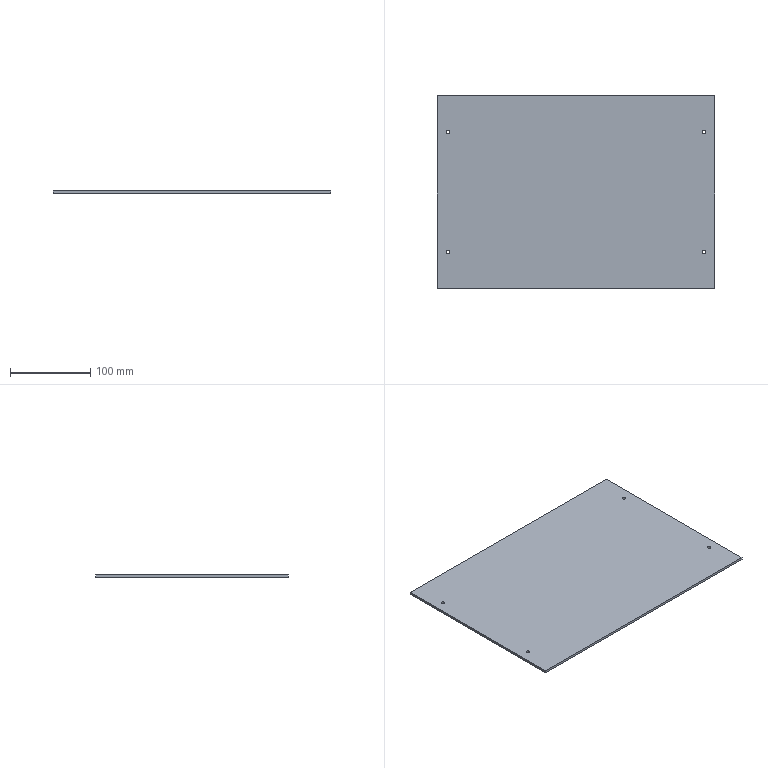Part | SolidWorks | features Cut 1, Extrusion 1 | 1 solid | 14 faces | box 346 x 240 x 3 mm | volume 248938 mm3 | cylinder 8 | plane 6 | commonest cylinder face diameters 4.4 x8
STEP:
#1=CARTESIAN_POINT('',(-162.2,-75.,0.));
#2=VERTEX_POINT('',#1);
#3=CARTESIAN_POINT('',(-157.8,-75.,0.));
#4=VERTEX_POINT('',#3);
#5=CARTESIAN_POINT('',(-160.,-75.,0.));
#6=DIRECTION('',(0.,0.,1.));
#7=DIRECTION('',(1.,0.,0.));
#8=AXIS2_PLACEMENT_3D('',#5,#6,#7);
#9=CIRCLE('',#8,2.2);
#10=EDGE_CURVE('',#2,#4,#9,.T.);
#11=ORIENTED_EDGE('',*,*,#10,.F.);
#12=CARTESIAN_POINT('',(-162.2,-75.,3.));
#13=VERTEX_POINT('',#12);
#14=CARTESIAN_POINT('',(-162.2,-75.,-7.));
#15=DIRECTION('',(0.,0.,1.));
#16=VECTOR('',#15,1000.);
#17=LINE('',#14,#16);
#18=EDGE_CURVE('',#2,#13,#17,.T.);
#19=ORIENTED_EDGE('',*,*,#18,.T.);
#20=CARTESIAN_POINT('',(-157.8,-75.,3.));
#21=VERTEX_POINT('',#20);
#22=CARTESIAN_POINT('',(-160.,-75.,3.));
#23=DIRECTION('',(0.,0.,1.));
#24=DIRECTION('',(1.,0.,0.));
#25=AXIS2_PLACEMENT_3D('',#22,#23,#24);
#26=CIRCLE('',#25,2.2);
#27=EDGE_CURVE('',#13,#21,#26,.T.);
#28=ORIENTED_EDGE('',*,*,#27,.T.);
#29=CARTESIAN_POINT('',(-157.8,-75.,-7.));
#30=DIRECTION('',(0.,0.,1.));
#31=VECTOR('',#30,1000.);
#32=LINE('',#29,#31);
#33=EDGE_CURVE('',#4,#21,#32,.T.);
#34=ORIENTED_EDGE('',*,*,#33,.F.);
#35=EDGE_LOOP('',(#11,#19,#28,#34));
#36=FACE_OUTER_BOUND('',#35,.T.);
#37=CARTESIAN_POINT('',(-160.,-75.,-7.));
#38=DIRECTION('',(0.,0.,1.));
#39=DIRECTION('',(1.,0.,0.));
#40=AXIS2_PLACEMENT_3D('',#37,#38,#39);
#41=CYLINDRICAL_SURFACE('',#40,2.2);
#42=ADVANCED_FACE('',(#36),#41,.F.);
#43=CARTESIAN_POINT('',(-162.2,75.,0.));
#44=VERTEX_POINT('',#43);
#45=CARTESIAN_POINT('',(-157.8,75.,0.));
#46=VERTEX_POINT('',#45);
#47=CARTESIAN_POINT('',(-160.,75.,0.));
#48=DIRECTION('',(0.,0.,1.));
#49=DIRECTION('',(1.,0.,0.));
#50=AXIS2_PLACEMENT_3D('',#47,#48,#49);
#51=CIRCLE('',#50,2.2);
#52=EDGE_CURVE('',#44,#46,#51,.T.);
#53=ORIENTED_EDGE('',*,*,#52,.F.);
#54=CARTESIAN_POINT('',(-162.2,75.,3.));
#55=VERTEX_POINT('',#54);
#56=CARTESIAN_POINT('',(-162.2,75.,-7.));
#57=DIRECTION('',(0.,0.,1.));
#58=VECTOR('',#57,1000.);
#59=LINE('',#56,#58);
#60=EDGE_CURVE('',#44,#55,#59,.T.);
#61=ORIENTED_EDGE('',*,*,#60,.T.);
#62=CARTESIAN_POINT('',(-157.8,75.,3.));
#63=VERTEX_POINT('',#62);
#64=CARTESIAN_POINT('',(-160.,75.,3.));
#65=DIRECTION('',(0.,0.,1.));
#66=DIRECTION('',(1.,0.,0.));
#67=AXIS2_PLACEMENT_3D('',#64,#65,#66);
#68=CIRCLE('',#67,2.2);
#69=EDGE_CURVE('',#55,#63,#68,.T.);
#70=ORIENTED_EDGE('',*,*,#69,.T.);
#71=CARTESIAN_POINT('',(-157.8,75.,-7.));
#72=DIRECTION('',(0.,0.,1.));
#73=VECTOR('',#72,1000.);
#74=LINE('',#71,#73);
#75=EDGE_CURVE('',#46,#63,#74,.T.);
#76=ORIENTED_EDGE('',*,*,#75,.F.);
#77=EDGE_LOOP('',(#53,#61,#70,#76));
#78=FACE_OUTER_BOUND('',#77,.T.);
#79=CARTESIAN_POINT('',(-160.,75.,-7.));
#80=DIRECTION('',(0.,0.,1.));
#81=DIRECTION('',(1.,0.,0.));
#82=AXIS2_PLACEMENT_3D('',#79,#80,#81);
#83=CYLINDRICAL_SURFACE('',#82,2.2);
#84=ADVANCED_FACE('',(#78),#83,.F.);
#85=CARTESIAN_POINT('',(157.8,-75.,0.));
#86=VERTEX_POINT('',#85);
#87=CARTESIAN_POINT('',(162.2,-75.,0.));
#88=VERTEX_POINT('',#87);
#89=CARTESIAN_POINT('',(160.,-75.,0.));
#90=DIRECTION('',(0.,0.,1.));
#91=DIRECTION('',(1.,0.,0.));
#92=AXIS2_PLACEMENT_3D('',#89,#90,#91);
#93=CIRCLE('',#92,2.2);
#94=EDGE_CURVE('',#86,#88,#93,.T.);
#95=ORIENTED_EDGE('',*,*,#94,.F.);
#96=CARTESIAN_POINT('',(157.8,-75.,3.));
#97=VERTEX_POINT('',#96);
#98=CARTESIAN_POINT('',(157.8,-75.,-7.));
#99=DIRECTION('',(0.,0.,1.));
#100=VECTOR('',#99,1000.);
#101=LINE('',#98,#100);
#102=EDGE_CURVE('',#86,#97,#101,.T.);
#103=ORIENTED_EDGE('',*,*,#102,.T.);
#104=CARTESIAN_POINT('',(162.2,-75.,3.));
#105=VERTEX_POINT('',#104);
#106=CARTESIAN_POINT('',(160.,-75.,3.));
#107=DIRECTION('',(0.,0.,1.));
#108=DIRECTION('',(1.,0.,0.));
#109=AXIS2_PLACEMENT_3D('',#106,#107,#108);
#110=CIRCLE('',#109,2.2);
#111=EDGE_CURVE('',#97,#105,#110,.T.);
#112=ORIENTED_EDGE('',*,*,#111,.T.);
#113=CARTESIAN_POINT('',(162.2,-75.,-7.));
#114=DIRECTION('',(0.,0.,1.));
#115=VECTOR('',#114,1000.);
#116=LINE('',#113,#115);
#117=EDGE_CURVE('',#88,#105,#116,.T.);
#118=ORIENTED_EDGE('',*,*,#117,.F.);
#119=EDGE_LOOP('',(#95,#103,#112,#118));
#120=FACE_OUTER_BOUND('',#119,.T.);
#121=CARTESIAN_POINT('',(160.,-75.,-7.));
#122=DIRECTION('',(0.,0.,1.));
#123=DIRECTION('',(1.,0.,0.));
#124=AXIS2_PLACEMENT_3D('',#121,#122,#123);
#125=CYLINDRICAL_SURFACE('',#124,2.2);
#126=ADVANCED_FACE('',(#120),#125,.F.);
#127=CARTESIAN_POINT('',(157.8,75.,0.));
#128=VERTEX_POINT('',#127);
#129=CARTESIAN_POINT('',(162.2,75.,0.));
#130=VERTEX_POINT('',#129);
#131=CARTESIAN_POINT('',(160.,75.,0.));
#132=DIRECTION('',(0.,0.,1.));
#133=DIRECTION('',(1.,0.,0.));
#134=AXIS2_PLACEMENT_3D('',#131,#132,#133);
#135=CIRCLE('',#134,2.2);
#136=EDGE_CURVE('',#128,#130,#135,.T.);
#137=ORIENTED_EDGE('',*,*,#136,.F.);
#138=CARTESIAN_POINT('',(157.8,75.,3.));
#139=VERTEX_POINT('',#138);
#140=CARTESIAN_POINT('',(157.8,75.,-7.));
#141=DIRECTION('',(0.,0.,1.));
#142=VECTOR('',#141,1000.);
#143=LINE('',#140,#142);
#144=EDGE_CURVE('',#128,#139,#143,.T.);
#145=ORIENTED_EDGE('',*,*,#144,.T.);
#146=CARTESIAN_POINT('',(162.2,75.,3.));
#147=VERTEX_POINT('',#146);
#148=CARTESIAN_POINT('',(160.,75.,3.));
#149=DIRECTION('',(0.,0.,1.));
#150=DIRECTION('',(1.,0.,0.));
#151=AXIS2_PLACEMENT_3D('',#148,#149,#150);
#152=CIRCLE('',#151,2.2);
#153=EDGE_CURVE('',#139,#147,#152,.T.);
#154=ORIENTED_EDGE('',*,*,#153,.T.);
#155=CARTESIAN_POINT('',(162.2,75.,-7.));
#156=DIRECTION('',(0.,0.,1.));
#157=VECTOR('',#156,1000.);
#158=LINE('',#155,#157);
#159=EDGE_CURVE('',#130,#147,#158,.T.);
#160=ORIENTED_EDGE('',*,*,#159,.F.);
#161=EDGE_LOOP('',(#137,#145,#154,#160));
#162=FACE_OUTER_BOUND('',#161,.T.);
#163=CARTESIAN_POINT('',(160.,75.,-7.));
#164=DIRECTION('',(0.,0.,1.));
#165=DIRECTION('',(1.,0.,0.));
#166=AXIS2_PLACEMENT_3D('',#163,#164,#165);
#167=CYLINDRICAL_SURFACE('',#166,2.2);
#168=ADVANCED_FACE('',(#162),#167,.F.);
#169=CARTESIAN_POINT('',(-173.,120.,0.));
#170=VERTEX_POINT('',#169);
#171=CARTESIAN_POINT('',(-173.,-120.,0.));
#172=VERTEX_POINT('',#171);
#173=CARTESIAN_POINT('',(-173.,-120.,0.));
#174=DIRECTION('',(0.,-1.,0.));
#175=VECTOR('',#174,1000.);
#176=LINE('',#173,#175);
#177=EDGE_CURVE('',#170,#172,#176,.T.);
#178=ORIENTED_EDGE('',*,*,#177,.T.);
#179=CARTESIAN_POINT('',(-173.,-120.,3.));
#180=VERTEX_POINT('',#179);
#181=CARTESIAN_POINT('',(-173.,-120.,3.));
#182=DIRECTION('',(0.,0.,-1.));
#183=VECTOR('',#182,1000.);
#184=LINE('',#181,#183);
#185=EDGE_CURVE('',#180,#172,#184,.T.);
#186=ORIENTED_EDGE('',*,*,#185,.F.);
#187=CARTESIAN_POINT('',(-173.,120.,3.));
#188=VERTEX_POINT('',#187);
#189=CARTESIAN_POINT('',(-173.,-120.,3.));
#190=DIRECTION('',(0.,-1.,0.));
#191=VECTOR('',#190,1000.);
#192=LINE('',#189,#191);
#193=EDGE_CURVE('',#188,#180,#192,.T.);
#194=ORIENTED_EDGE('',*,*,#193,.F.);
#195=CARTESIAN_POINT('',(-173.,120.,3.));
#196=DIRECTION('',(0.,0.,-1.));
#197=VECTOR('',#196,1000.);
#198=LINE('',#195,#197);
#199=EDGE_CURVE('',#188,#170,#198,.T.);
#200=ORIENTED_EDGE('',*,*,#199,.T.);
#201=EDGE_LOOP('',(#178,#186,#194,#200));
#202=FACE_OUTER_BOUND('',#201,.T.);
#203=CARTESIAN_POINT('',(-173.,-120.,3.));
#204=DIRECTION('',(1.,0.,0.));
#205=DIRECTION('',(0.,0.,-1.));
#206=AXIS2_PLACEMENT_3D('',#203,#204,#205);
#207=PLANE('',#206);
#208=ADVANCED_FACE('',(#202),#207,.F.);
#209=CARTESIAN_POINT('',(173.,-120.,0.));
#210=VERTEX_POINT('',#209);
#211=CARTESIAN_POINT('',(173.,-120.,0.));
#212=DIRECTION('',(1.,0.,0.));
#213=VECTOR('',#212,1000.);
#214=LINE('',#211,#213);
#215=EDGE_CURVE('',#172,#210,#214,.T.);
#216=ORIENTED_EDGE('',*,*,#215,.T.);
#217=CARTESIAN_POINT('',(173.,-120.,3.));
#218=VERTEX_POINT('',#217);
#219=CARTESIAN_POINT('',(173.,-120.,3.));
#220=DIRECTION('',(0.,0.,-1.));
#221=VECTOR('',#220,1000.);
#222=LINE('',#219,#221);
#223=EDGE_CURVE('',#218,#210,#222,.T.);
#224=ORIENTED_EDGE('',*,*,#223,.F.);
#225=CARTESIAN_POINT('',(173.,-120.,3.));
#226=DIRECTION('',(1.,0.,0.));
#227=VECTOR('',#226,1000.);
#228=LINE('',#225,#227);
#229=EDGE_CURVE('',#180,#218,#228,.T.);
#230=ORIENTED_EDGE('',*,*,#229,.F.);
#231=ORIENTED_EDGE('',*,*,#185,.T.);
#232=EDGE_LOOP('',(#216,#224,#230,#231));
#233=FACE_OUTER_BOUND('',#232,.T.);
#234=CARTESIAN_POINT('',(173.,-120.,3.));
#235=DIRECTION('',(0.,1.,0.));
#236=DIRECTION('',(-1.,0.,0.));
#237=AXIS2_PLACEMENT_3D('',#234,#235,#236);
#238=PLANE('',#237);
#239=ADVANCED_FACE('',(#233),#238,.F.);
#240=CARTESIAN_POINT('',(173.,120.,0.));
#241=VERTEX_POINT('',#240);
#242=CARTESIAN_POINT('',(173.,-120.,0.));
#243=DIRECTION('',(0.,1.,0.));
#244=VECTOR('',#243,1000.);
#245=LINE('',#242,#244);
#246=EDGE_CURVE('',#210,#241,#245,.T.);
#247=ORIENTED_EDGE('',*,*,#246,.T.);
#248=CARTESIAN_POINT('',(173.,120.,3.));
#249=VERTEX_POINT('',#248);
#250=CARTESIAN_POINT('',(173.,120.,3.));
#251=DIRECTION('',(0.,0.,-1.));
#252=VECTOR('',#251,1000.);
#253=LINE('',#250,#252);
#254=EDGE_CURVE('',#249,#241,#253,.T.);
#255=ORIENTED_EDGE('',*,*,#254,.F.);
#256=CARTESIAN_POINT('',(173.,-120.,3.));
#257=DIRECTION('',(0.,1.,0.));
#258=VECTOR('',#257,1000.);
#259=LINE('',#256,#258);
#260=EDGE_CURVE('',#218,#249,#259,.T.);
#261=ORIENTED_EDGE('',*,*,#260,.F.);
#262=ORIENTED_EDGE('',*,*,#223,.T.);
#263=EDGE_LOOP('',(#247,#255,#261,#262));
#264=FACE_OUTER_BOUND('',#263,.T.);
#265=CARTESIAN_POINT('',(173.,-120.,3.));
#266=DIRECTION('',(-1.,0.,0.));
#267=DIRECTION('',(0.,0.,1.));
#268=AXIS2_PLACEMENT_3D('',#265,#266,#267);
#269=PLANE('',#268);
#270=ADVANCED_FACE('',(#264),#269,.F.);
#271=CARTESIAN_POINT('',(173.,120.,0.));
#272=DIRECTION('',(-1.,0.,0.));
#273=VECTOR('',#272,1000.);
#274=LINE('',#271,#273);
#275=EDGE_CURVE('',#241,#170,#274,.T.);
#276=ORIENTED_EDGE('',*,*,#275,.T.);
#277=ORIENTED_EDGE('',*,*,#199,.F.);
#278=CARTESIAN_POINT('',(173.,120.,3.));
#279=DIRECTION('',(-1.,0.,0.));
#280=VECTOR('',#279,1000.);
#281=LINE('',#278,#280);
#282=EDGE_CURVE('',#249,#188,#281,.T.);
#283=ORIENTED_EDGE('',*,*,#282,.F.);
#284=ORIENTED_EDGE('',*,*,#254,.T.);
#285=EDGE_LOOP('',(#276,#277,#283,#284));
#286=FACE_OUTER_BOUND('',#285,.T.);
#287=CARTESIAN_POINT('',(173.,120.,3.));
#288=DIRECTION('',(0.,-1.,0.));
#289=DIRECTION('',(1.,0.,0.));
#290=AXIS2_PLACEMENT_3D('',#287,#288,#289);
#291=PLANE('',#290);
#292=ADVANCED_FACE('',(#286),#291,.F.);
#293=CARTESIAN_POINT('',(-160.,-75.,3.));
#294=DIRECTION('',(0.,0.,1.));
#295=DIRECTION('',(1.,0.,0.));
#296=AXIS2_PLACEMENT_3D('',#293,#294,#295);
#297=CIRCLE('',#296,2.2);
#298=EDGE_CURVE('',#21,#13,#297,.T.);
#299=ORIENTED_EDGE('',*,*,#298,.F.);
#300=ORIENTED_EDGE('',*,*,#27,.F.);
#301=EDGE_LOOP('',(#299,#300));
#302=FACE_BOUND('',#301,.T.);
#303=CARTESIAN_POINT('',(-160.,75.,3.));
#304=DIRECTION('',(0.,0.,1.));
#305=DIRECTION('',(1.,0.,0.));
#306=AXIS2_PLACEMENT_3D('',#303,#304,#305);
#307=CIRCLE('',#306,2.2);
#308=EDGE_CURVE('',#63,#55,#307,.T.);
#309=ORIENTED_EDGE('',*,*,#308,.F.);
#310=ORIENTED_EDGE('',*,*,#69,.F.);
#311=EDGE_LOOP('',(#309,#310));
#312=FACE_BOUND('',#311,.T.);
#313=CARTESIAN_POINT('',(160.,-75.,3.));
#314=DIRECTION('',(0.,0.,1.));
#315=DIRECTION('',(1.,0.,0.));
#316=AXIS2_PLACEMENT_3D('',#313,#314,#315);
#317=CIRCLE('',#316,2.2);
#318=EDGE_CURVE('',#105,#97,#317,.T.);
#319=ORIENTED_EDGE('',*,*,#318,.F.);
#320=ORIENTED_EDGE('',*,*,#111,.F.);
#321=EDGE_LOOP('',(#319,#320));
#322=FACE_BOUND('',#321,.T.);
#323=CARTESIAN_POINT('',(160.,75.,3.));
#324=DIRECTION('',(0.,0.,1.));
#325=DIRECTION('',(1.,0.,0.));
#326=AXIS2_PLACEMENT_3D('',#323,#324,#325);
#327=CIRCLE('',#326,2.2);
#328=EDGE_CURVE('',#147,#139,#327,.T.);
#329=ORIENTED_EDGE('',*,*,#328,.F.);
#330=ORIENTED_EDGE('',*,*,#153,.F.);
#331=EDGE_LOOP('',(#329,#330));
#332=FACE_BOUND('',#331,.T.);
#333=ORIENTED_EDGE('',*,*,#193,.T.);
#334=ORIENTED_EDGE('',*,*,#229,.T.);
#335=ORIENTED_EDGE('',*,*,#260,.T.);
#336=ORIENTED_EDGE('',*,*,#282,.T.);
#337=EDGE_LOOP('',(#333,#334,#335,#336));
#338=FACE_OUTER_BOUND('',#337,.T.);
#339=CARTESIAN_POINT('',(0.,0.,3.));
#340=DIRECTION('',(0.,0.,1.));
#341=DIRECTION('',(1.,0.,0.));
#342=AXIS2_PLACEMENT_3D('',#339,#340,#341);
#343=PLANE('',#342);
#344=ADVANCED_FACE('',(#302,#312,#322,#332,#338),#343,.T.);
#345=CARTESIAN_POINT('',(-160.,-75.,0.));
#346=DIRECTION('',(0.,0.,1.));
#347=DIRECTION('',(1.,0.,0.));
#348=AXIS2_PLACEMENT_3D('',#345,#346,#347);
#349=CIRCLE('',#348,2.2);
#350=EDGE_CURVE('',#4,#2,#349,.T.);
#351=ORIENTED_EDGE('',*,*,#350,.T.);
#352=ORIENTED_EDGE('',*,*,#10,.T.);
#353=EDGE_LOOP('',(#351,#352));
#354=FACE_BOUND('',#353,.T.);
#355=CARTESIAN_POINT('',(-160.,75.,0.));
#356=DIRECTION('',(0.,0.,1.));
#357=DIRECTION('',(1.,0.,0.));
#358=AXIS2_PLACEMENT_3D('',#355,#356,#357);
#359=CIRCLE('',#358,2.2);
#360=EDGE_CURVE('',#46,#44,#359,.T.);
#361=ORIENTED_EDGE('',*,*,#360,.T.);
#362=ORIENTED_EDGE('',*,*,#52,.T.);
#363=EDGE_LOOP('',(#361,#362));
#364=FACE_BOUND('',#363,.T.);
#365=CARTESIAN_POINT('',(160.,-75.,0.));
#366=DIRECTION('',(0.,0.,1.));
#367=DIRECTION('',(1.,0.,0.));
#368=AXIS2_PLACEMENT_3D('',#365,#366,#367);
#369=CIRCLE('',#368,2.2);
#370=EDGE_CURVE('',#88,#86,#369,.T.);
#371=ORIENTED_EDGE('',*,*,#370,.T.);
#372=ORIENTED_EDGE('',*,*,#94,.T.);
#373=EDGE_LOOP('',(#371,#372));
#374=FACE_BOUND('',#373,.T.);
#375=CARTESIAN_POINT('',(160.,75.,0.));
#376=DIRECTION('',(0.,0.,1.));
#377=DIRECTION('',(1.,0.,0.));
#378=AXIS2_PLACEMENT_3D('',#375,#376,#377);
#379=CIRCLE('',#378,2.2);
#380=EDGE_CURVE('',#130,#128,#379,.T.);
#381=ORIENTED_EDGE('',*,*,#380,.T.);
#382=ORIENTED_EDGE('',*,*,#136,.T.);
#383=EDGE_LOOP('',(#381,#382));
#384=FACE_BOUND('',#383,.T.);
#385=ORIENTED_EDGE('',*,*,#177,.F.);
#386=ORIENTED_EDGE('',*,*,#275,.F.);
#387=ORIENTED_EDGE('',*,*,#246,.F.);
#388=ORIENTED_EDGE('',*,*,#215,.F.);
#389=EDGE_LOOP('',(#385,#386,#387,#388));
#390=FACE_OUTER_BOUND('',#389,.T.);
#391=CARTESIAN_POINT('',(0.,0.,0.));
#392=DIRECTION('',(0.,0.,1.));
#393=DIRECTION('',(1.,0.,0.));
#394=AXIS2_PLACEMENT_3D('',#391,#392,#393);
#395=PLANE('',#394);
#396=ADVANCED_FACE('',(#354,#364,#374,#384,#390),#395,.F.);
#397=ORIENTED_EDGE('',*,*,#144,.F.);
#398=ORIENTED_EDGE('',*,*,#380,.F.);
#399=ORIENTED_EDGE('',*,*,#159,.T.);
#400=ORIENTED_EDGE('',*,*,#328,.T.);
#401=EDGE_LOOP('',(#397,#398,#399,#400));
#402=FACE_OUTER_BOUND('',#401,.T.);
#403=CARTESIAN_POINT('',(160.,75.,-7.));
#404=DIRECTION('',(0.,0.,1.));
#405=DIRECTION('',(1.,0.,0.));
#406=AXIS2_PLACEMENT_3D('',#403,#404,#405);
#407=CYLINDRICAL_SURFACE('',#406,2.2);
#408=ADVANCED_FACE('',(#402),#407,.F.);
#409=ORIENTED_EDGE('',*,*,#102,.F.);
#410=ORIENTED_EDGE('',*,*,#370,.F.);
#411=ORIENTED_EDGE('',*,*,#117,.T.);
#412=ORIENTED_EDGE('',*,*,#318,.T.);
#413=EDGE_LOOP('',(#409,#410,#411,#412));
#414=FACE_OUTER_BOUND('',#413,.T.);
#415=CARTESIAN_POINT('',(160.,-75.,-7.));
#416=DIRECTION('',(0.,0.,1.));
#417=DIRECTION('',(1.,0.,0.));
#418=AXIS2_PLACEMENT_3D('',#415,#416,#417);
#419=CYLINDRICAL_SURFACE('',#418,2.2);
#420=ADVANCED_FACE('',(#414),#419,.F.);
#421=ORIENTED_EDGE('',*,*,#60,.F.);
#422=ORIENTED_EDGE('',*,*,#360,.F.);
#423=ORIENTED_EDGE('',*,*,#75,.T.);
#424=ORIENTED_EDGE('',*,*,#308,.T.);
#425=EDGE_LOOP('',(#421,#422,#423,#424));
#426=FACE_OUTER_BOUND('',#425,.T.);
#427=CARTESIAN_POINT('',(-160.,75.,-7.));
#428=DIRECTION('',(0.,0.,1.));
#429=DIRECTION('',(1.,0.,0.));
#430=AXIS2_PLACEMENT_3D('',#427,#428,#429);
#431=CYLINDRICAL_SURFACE('',#430,2.2);
#432=ADVANCED_FACE('',(#426),#431,.F.);
#433=ORIENTED_EDGE('',*,*,#18,.F.);
#434=ORIENTED_EDGE('',*,*,#350,.F.);
#435=ORIENTED_EDGE('',*,*,#33,.T.);
#436=ORIENTED_EDGE('',*,*,#298,.T.);
#437=EDGE_LOOP('',(#433,#434,#435,#436));
#438=FACE_OUTER_BOUND('',#437,.T.);
#439=CARTESIAN_POINT('',(-160.,-75.,-7.));
#440=DIRECTION('',(0.,0.,1.));
#441=DIRECTION('',(1.,0.,0.));
#442=AXIS2_PLACEMENT_3D('',#439,#440,#441);
#443=CYLINDRICAL_SURFACE('',#442,2.2);
#444=ADVANCED_FACE('',(#438),#443,.F.);
#445=CLOSED_SHELL('',(#42,#84,#126,#168,#208,#239,#270,#292,#344,#396,#408,#420,#432,#444));
#446=MANIFOLD_SOLID_BREP('',#445);
#447=CARTESIAN_POINT('',(0.,0.,0.));
#448=DIRECTION('',(0.,0.,1.));
#449=DIRECTION('',(1.,0.,0.));
#450=AXIS2_PLACEMENT_3D('',#447,#448,#449);
#451=(LENGTH_UNIT()NAMED_UNIT(*)SI_UNIT(.MILLI.,.METRE.));
#452=UNCERTAINTY_MEASURE_WITH_UNIT(LENGTH_MEASURE(0.00001),#451,'','');
#453=(NAMED_UNIT(*)PLANE_ANGLE_UNIT()SI_UNIT($,.RADIAN.));
#454=(NAMED_UNIT(*)SI_UNIT($,.STERADIAN.)SOLID_ANGLE_UNIT());
#455=(GEOMETRIC_REPRESENTATION_CONTEXT(3)GLOBAL_UNCERTAINTY_ASSIGNED_CONTEXT((#452))GLOBAL_UNIT_ASSIGNED_CONTEXT((#451,#453,#454))REPRESENTATION_CONTEXT('',''));
#456=ADVANCED_BREP_SHAPE_REPRESENTATION('',(#446,#450),#455);